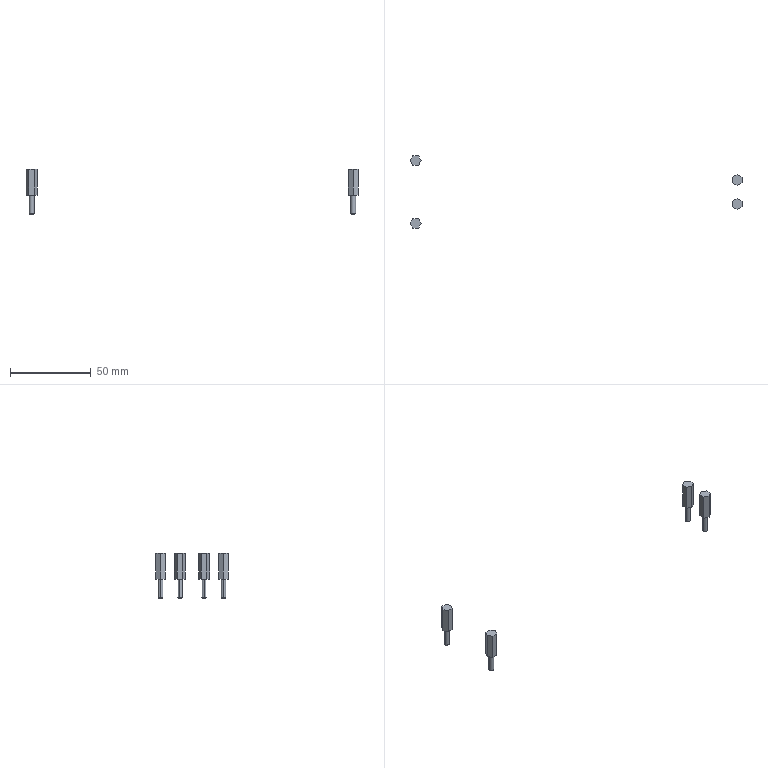Part | SolidWorks | features Chamfer 4, Extrusion 1, ICE 1 | 4 solids | 52 faces | box 205.964 x 45 x 28 mm | volume 2330 mm3 | plane 36 | cone 8 | cylinder 8 | commonest cylinder face diameters 3 x8
STEP:
#1=CARTESIAN_POINT('',(-83.5,19.5,-12.));
#2=VERTEX_POINT('',#1);
#3=CARTESIAN_POINT('',(-81.5,19.5,-12.));
#4=VERTEX_POINT('',#3);
#5=CARTESIAN_POINT('',(-82.5,19.5,-12.));
#6=DIRECTION('',(0.,0.,-1.));
#7=DIRECTION('',(1.,0.,0.));
#8=AXIS2_PLACEMENT_3D('',#5,#6,#7);
#9=CIRCLE('',#8,1.);
#10=EDGE_CURVE('',#2,#4,#9,.T.);
#11=ORIENTED_EDGE('',*,*,#10,.F.);
#12=CARTESIAN_POINT('',(-84.,19.5,-11.5));
#13=VERTEX_POINT('',#12);
#14=CARTESIAN_POINT('',(-84.,19.5,-11.5));
#15=DIRECTION('',(-0.7071,0.,0.7071));
#16=VECTOR('',#15,1000.);
#17=LINE('',#14,#16);
#18=EDGE_CURVE('',#2,#13,#17,.T.);
#19=ORIENTED_EDGE('',*,*,#18,.T.);
#20=CARTESIAN_POINT('',(-81.,19.5,-11.5));
#21=VERTEX_POINT('',#20);
#22=CARTESIAN_POINT('',(-82.5,19.5,-11.5));
#23=DIRECTION('',(0.,0.,1.));
#24=DIRECTION('',(1.,0.,0.));
#25=AXIS2_PLACEMENT_3D('',#22,#23,#24);
#26=CIRCLE('',#25,1.5);
#27=EDGE_CURVE('',#21,#13,#26,.T.);
#28=ORIENTED_EDGE('',*,*,#27,.F.);
#29=CARTESIAN_POINT('',(-81.,19.5,-11.5));
#30=DIRECTION('',(0.7071,0.,0.7071));
#31=VECTOR('',#30,1000.);
#32=LINE('',#29,#31);
#33=EDGE_CURVE('',#4,#21,#32,.T.);
#34=ORIENTED_EDGE('',*,*,#33,.F.);
#35=EDGE_LOOP('',(#11,#19,#28,#34));
#36=FACE_OUTER_BOUND('',#35,.T.);
#37=CARTESIAN_POINT('',(-82.5,19.5,-11.5));
#38=DIRECTION('',(0.,0.,1.));
#39=DIRECTION('',(1.,0.,0.));
#40=AXIS2_PLACEMENT_3D('',#37,#38,#39);
#41=CONICAL_SURFACE('',#40,1.5,0.7854);
#42=ADVANCED_FACE('',(#36),#41,.T.);
#43=ORIENTED_EDGE('',*,*,#27,.T.);
#44=CARTESIAN_POINT('',(-84.,19.5,0.));
#45=VERTEX_POINT('',#44);
#46=CARTESIAN_POINT('',(-84.,19.5,-12.));
#47=DIRECTION('',(0.,0.,1.));
#48=VECTOR('',#47,1000.);
#49=LINE('',#46,#48);
#50=EDGE_CURVE('',#13,#45,#49,.T.);
#51=ORIENTED_EDGE('',*,*,#50,.T.);
#52=CARTESIAN_POINT('',(-81.,19.5,0.));
#53=VERTEX_POINT('',#52);
#54=CARTESIAN_POINT('',(-82.5,19.5,0.));
#55=DIRECTION('',(0.,0.,1.));
#56=DIRECTION('',(1.,0.,0.));
#57=AXIS2_PLACEMENT_3D('',#54,#55,#56);
#58=CIRCLE('',#57,1.5);
#59=EDGE_CURVE('',#53,#45,#58,.T.);
#60=ORIENTED_EDGE('',*,*,#59,.F.);
#61=CARTESIAN_POINT('',(-81.,19.5,-12.));
#62=DIRECTION('',(0.,0.,1.));
#63=VECTOR('',#62,1000.);
#64=LINE('',#61,#63);
#65=EDGE_CURVE('',#21,#53,#64,.T.);
#66=ORIENTED_EDGE('',*,*,#65,.F.);
#67=EDGE_LOOP('',(#43,#51,#60,#66));
#68=FACE_OUTER_BOUND('',#67,.T.);
#69=CARTESIAN_POINT('',(-82.5,19.5,-12.));
#70=DIRECTION('',(0.,0.,1.));
#71=DIRECTION('',(1.,0.,0.));
#72=AXIS2_PLACEMENT_3D('',#69,#70,#71);
#73=CYLINDRICAL_SURFACE('',#72,1.5);
#74=ADVANCED_FACE('',(#68),#73,.T.);
#75=CARTESIAN_POINT('',(-84.232,16.5,0.));
#76=VERTEX_POINT('',#75);
#77=CARTESIAN_POINT('',(-85.964,19.5,0.));
#78=VERTEX_POINT('',#77);
#79=CARTESIAN_POINT('',(-84.232,16.5,0.));
#80=DIRECTION('',(-0.5,0.866,0.));
#81=VECTOR('',#80,1000.);
#82=LINE('',#79,#81);
#83=EDGE_CURVE('',#76,#78,#82,.T.);
#84=ORIENTED_EDGE('',*,*,#83,.F.);
#85=CARTESIAN_POINT('',(-84.232,16.5,16.));
#86=VERTEX_POINT('',#85);
#87=CARTESIAN_POINT('',(-84.232,16.5,16.));
#88=DIRECTION('',(0.,0.,-1.));
#89=VECTOR('',#88,1000.);
#90=LINE('',#87,#89);
#91=EDGE_CURVE('',#86,#76,#90,.T.);
#92=ORIENTED_EDGE('',*,*,#91,.F.);
#93=CARTESIAN_POINT('',(-85.964,19.5,16.));
#94=VERTEX_POINT('',#93);
#95=CARTESIAN_POINT('',(-84.232,16.5,16.));
#96=DIRECTION('',(-0.5,0.866,0.));
#97=VECTOR('',#96,1000.);
#98=LINE('',#95,#97);
#99=EDGE_CURVE('',#86,#94,#98,.T.);
#100=ORIENTED_EDGE('',*,*,#99,.T.);
#101=CARTESIAN_POINT('',(-85.964,19.5,16.));
#102=DIRECTION('',(0.,0.,-1.));
#103=VECTOR('',#102,1000.);
#104=LINE('',#101,#103);
#105=EDGE_CURVE('',#94,#78,#104,.T.);
#106=ORIENTED_EDGE('',*,*,#105,.T.);
#107=EDGE_LOOP('',(#84,#92,#100,#106));
#108=FACE_OUTER_BOUND('',#107,.T.);
#109=CARTESIAN_POINT('',(-84.232,16.5,16.));
#110=DIRECTION('',(-0.866,-0.5,0.));
#111=DIRECTION('',(0.5,-0.866,0.));
#112=AXIS2_PLACEMENT_3D('',#109,#110,#111);
#113=PLANE('',#112);
#114=ADVANCED_FACE('',(#108),#113,.T.);
#115=CARTESIAN_POINT('',(-80.768,16.5,0.));
#116=VERTEX_POINT('',#115);
#117=CARTESIAN_POINT('',(-80.768,16.5,0.));
#118=DIRECTION('',(-1.,0.,0.));
#119=VECTOR('',#118,1000.);
#120=LINE('',#117,#119);
#121=EDGE_CURVE('',#116,#76,#120,.T.);
#122=ORIENTED_EDGE('',*,*,#121,.F.);
#123=CARTESIAN_POINT('',(-80.768,16.5,16.));
#124=VERTEX_POINT('',#123);
#125=CARTESIAN_POINT('',(-80.768,16.5,16.));
#126=DIRECTION('',(0.,0.,-1.));
#127=VECTOR('',#126,1000.);
#128=LINE('',#125,#127);
#129=EDGE_CURVE('',#124,#116,#128,.T.);
#130=ORIENTED_EDGE('',*,*,#129,.F.);
#131=CARTESIAN_POINT('',(-80.768,16.5,16.));
#132=DIRECTION('',(-1.,0.,0.));
#133=VECTOR('',#132,1000.);
#134=LINE('',#131,#133);
#135=EDGE_CURVE('',#124,#86,#134,.T.);
#136=ORIENTED_EDGE('',*,*,#135,.T.);
#137=ORIENTED_EDGE('',*,*,#91,.T.);
#138=EDGE_LOOP('',(#122,#130,#136,#137));
#139=FACE_OUTER_BOUND('',#138,.T.);
#140=CARTESIAN_POINT('',(-80.768,16.5,16.));
#141=DIRECTION('',(0.,-1.,0.));
#142=DIRECTION('',(0.,0.,-1.));
#143=AXIS2_PLACEMENT_3D('',#140,#141,#142);
#144=PLANE('',#143);
#145=ADVANCED_FACE('',(#139),#144,.T.);
#146=CARTESIAN_POINT('',(-79.036,19.5,0.));
#147=VERTEX_POINT('',#146);
#148=CARTESIAN_POINT('',(-79.036,19.5,0.));
#149=DIRECTION('',(-0.5,-0.866,0.));
#150=VECTOR('',#149,1000.);
#151=LINE('',#148,#150);
#152=EDGE_CURVE('',#147,#116,#151,.T.);
#153=ORIENTED_EDGE('',*,*,#152,.F.);
#154=CARTESIAN_POINT('',(-79.036,19.5,16.));
#155=VERTEX_POINT('',#154);
#156=CARTESIAN_POINT('',(-79.036,19.5,16.));
#157=DIRECTION('',(0.,0.,-1.));
#158=VECTOR('',#157,1000.);
#159=LINE('',#156,#158);
#160=EDGE_CURVE('',#155,#147,#159,.T.);
#161=ORIENTED_EDGE('',*,*,#160,.F.);
#162=CARTESIAN_POINT('',(-79.036,19.5,16.));
#163=DIRECTION('',(-0.5,-0.866,0.));
#164=VECTOR('',#163,1000.);
#165=LINE('',#162,#164);
#166=EDGE_CURVE('',#155,#124,#165,.T.);
#167=ORIENTED_EDGE('',*,*,#166,.T.);
#168=ORIENTED_EDGE('',*,*,#129,.T.);
#169=EDGE_LOOP('',(#153,#161,#167,#168));
#170=FACE_OUTER_BOUND('',#169,.T.);
#171=CARTESIAN_POINT('',(-79.036,19.5,16.));
#172=DIRECTION('',(0.866,-0.5,0.));
#173=DIRECTION('',(0.5,0.866,0.));
#174=AXIS2_PLACEMENT_3D('',#171,#172,#173);
#175=PLANE('',#174);
#176=ADVANCED_FACE('',(#170),#175,.T.);
#177=CARTESIAN_POINT('',(-80.768,22.5,0.));
#178=VERTEX_POINT('',#177);
#179=CARTESIAN_POINT('',(-80.768,22.5,0.));
#180=DIRECTION('',(0.5,-0.866,0.));
#181=VECTOR('',#180,1000.);
#182=LINE('',#179,#181);
#183=EDGE_CURVE('',#178,#147,#182,.T.);
#184=ORIENTED_EDGE('',*,*,#183,.F.);
#185=CARTESIAN_POINT('',(-80.768,22.5,16.));
#186=VERTEX_POINT('',#185);
#187=CARTESIAN_POINT('',(-80.768,22.5,16.));
#188=DIRECTION('',(0.,0.,-1.));
#189=VECTOR('',#188,1000.);
#190=LINE('',#187,#189);
#191=EDGE_CURVE('',#186,#178,#190,.T.);
#192=ORIENTED_EDGE('',*,*,#191,.F.);
#193=CARTESIAN_POINT('',(-80.768,22.5,16.));
#194=DIRECTION('',(0.5,-0.866,0.));
#195=VECTOR('',#194,1000.);
#196=LINE('',#193,#195);
#197=EDGE_CURVE('',#186,#155,#196,.T.);
#198=ORIENTED_EDGE('',*,*,#197,.T.);
#199=ORIENTED_EDGE('',*,*,#160,.T.);
#200=EDGE_LOOP('',(#184,#192,#198,#199));
#201=FACE_OUTER_BOUND('',#200,.T.);
#202=CARTESIAN_POINT('',(-80.768,22.5,16.));
#203=DIRECTION('',(0.866,0.5,0.));
#204=DIRECTION('',(-0.5,0.866,0.));
#205=AXIS2_PLACEMENT_3D('',#202,#203,#204);
#206=PLANE('',#205);
#207=ADVANCED_FACE('',(#201),#206,.T.);
#208=CARTESIAN_POINT('',(-84.232,22.5,0.));
#209=VERTEX_POINT('',#208);
#210=CARTESIAN_POINT('',(-84.232,22.5,0.));
#211=DIRECTION('',(1.,0.,0.));
#212=VECTOR('',#211,1000.);
#213=LINE('',#210,#212);
#214=EDGE_CURVE('',#209,#178,#213,.T.);
#215=ORIENTED_EDGE('',*,*,#214,.F.);
#216=CARTESIAN_POINT('',(-84.232,22.5,16.));
#217=VERTEX_POINT('',#216);
#218=CARTESIAN_POINT('',(-84.232,22.5,16.));
#219=DIRECTION('',(0.,0.,-1.));
#220=VECTOR('',#219,1000.);
#221=LINE('',#218,#220);
#222=EDGE_CURVE('',#217,#209,#221,.T.);
#223=ORIENTED_EDGE('',*,*,#222,.F.);
#224=CARTESIAN_POINT('',(-84.232,22.5,16.));
#225=DIRECTION('',(1.,0.,0.));
#226=VECTOR('',#225,1000.);
#227=LINE('',#224,#226);
#228=EDGE_CURVE('',#217,#186,#227,.T.);
#229=ORIENTED_EDGE('',*,*,#228,.T.);
#230=ORIENTED_EDGE('',*,*,#191,.T.);
#231=EDGE_LOOP('',(#215,#223,#229,#230));
#232=FACE_OUTER_BOUND('',#231,.T.);
#233=CARTESIAN_POINT('',(-84.232,22.5,16.));
#234=DIRECTION('',(0.,1.,0.));
#235=DIRECTION('',(0.,0.,1.));
#236=AXIS2_PLACEMENT_3D('',#233,#234,#235);
#237=PLANE('',#236);
#238=ADVANCED_FACE('',(#232),#237,.T.);
#239=CARTESIAN_POINT('',(-85.964,19.5,0.));
#240=DIRECTION('',(0.5,0.866,0.));
#241=VECTOR('',#240,1000.);
#242=LINE('',#239,#241);
#243=EDGE_CURVE('',#78,#209,#242,.T.);
#244=ORIENTED_EDGE('',*,*,#243,.F.);
#245=ORIENTED_EDGE('',*,*,#105,.F.);
#246=CARTESIAN_POINT('',(-85.964,19.5,16.));
#247=DIRECTION('',(0.5,0.866,0.));
#248=VECTOR('',#247,1000.);
#249=LINE('',#246,#248);
#250=EDGE_CURVE('',#94,#217,#249,.T.);
#251=ORIENTED_EDGE('',*,*,#250,.T.);
#252=ORIENTED_EDGE('',*,*,#222,.T.);
#253=EDGE_LOOP('',(#244,#245,#251,#252));
#254=FACE_OUTER_BOUND('',#253,.T.);
#255=CARTESIAN_POINT('',(-85.964,19.5,16.));
#256=DIRECTION('',(-0.866,0.5,0.));
#257=DIRECTION('',(-0.5,-0.866,0.));
#258=AXIS2_PLACEMENT_3D('',#255,#256,#257);
#259=PLANE('',#258);
#260=ADVANCED_FACE('',(#254),#259,.T.);
#261=ORIENTED_EDGE('',*,*,#99,.F.);
#262=ORIENTED_EDGE('',*,*,#135,.F.);
#263=ORIENTED_EDGE('',*,*,#166,.F.);
#264=ORIENTED_EDGE('',*,*,#197,.F.);
#265=ORIENTED_EDGE('',*,*,#228,.F.);
#266=ORIENTED_EDGE('',*,*,#250,.F.);
#267=EDGE_LOOP('',(#261,#262,#263,#264,#265,#266));
#268=FACE_OUTER_BOUND('',#267,.T.);
#269=CARTESIAN_POINT('',(0.,0.,16.));
#270=DIRECTION('',(0.,0.,-1.));
#271=DIRECTION('',(-1.,0.,0.));
#272=AXIS2_PLACEMENT_3D('',#269,#270,#271);
#273=PLANE('',#272);
#274=ADVANCED_FACE('',(#268),#273,.F.);
#275=ORIENTED_EDGE('',*,*,#59,.T.);
#276=CARTESIAN_POINT('',(-82.5,19.5,0.));
#277=DIRECTION('',(0.,0.,1.));
#278=DIRECTION('',(1.,0.,0.));
#279=AXIS2_PLACEMENT_3D('',#276,#277,#278);
#280=CIRCLE('',#279,1.5);
#281=EDGE_CURVE('',#45,#53,#280,.T.);
#282=ORIENTED_EDGE('',*,*,#281,.T.);
#283=EDGE_LOOP('',(#275,#282));
#284=FACE_BOUND('',#283,.T.);
#285=ORIENTED_EDGE('',*,*,#83,.T.);
#286=ORIENTED_EDGE('',*,*,#243,.T.);
#287=ORIENTED_EDGE('',*,*,#214,.T.);
#288=ORIENTED_EDGE('',*,*,#183,.T.);
#289=ORIENTED_EDGE('',*,*,#152,.T.);
#290=ORIENTED_EDGE('',*,*,#121,.T.);
#291=EDGE_LOOP('',(#285,#286,#287,#288,#289,#290));
#292=FACE_OUTER_BOUND('',#291,.T.);
#293=CARTESIAN_POINT('',(0.,0.,0.));
#294=DIRECTION('',(0.,0.,-1.));
#295=DIRECTION('',(-1.,0.,0.));
#296=AXIS2_PLACEMENT_3D('',#293,#294,#295);
#297=PLANE('',#296);
#298=ADVANCED_FACE('',(#284,#292),#297,.T.);
#299=ORIENTED_EDGE('',*,*,#50,.F.);
#300=CARTESIAN_POINT('',(-82.5,19.5,-11.5));
#301=DIRECTION('',(0.,0.,1.));
#302=DIRECTION('',(1.,0.,0.));
#303=AXIS2_PLACEMENT_3D('',#300,#301,#302);
#304=CIRCLE('',#303,1.5);
#305=EDGE_CURVE('',#13,#21,#304,.T.);
#306=ORIENTED_EDGE('',*,*,#305,.T.);
#307=ORIENTED_EDGE('',*,*,#65,.T.);
#308=ORIENTED_EDGE('',*,*,#281,.F.);
#309=EDGE_LOOP('',(#299,#306,#307,#308));
#310=FACE_OUTER_BOUND('',#309,.T.);
#311=CARTESIAN_POINT('',(-82.5,19.5,-12.));
#312=DIRECTION('',(0.,0.,1.));
#313=DIRECTION('',(1.,0.,0.));
#314=AXIS2_PLACEMENT_3D('',#311,#312,#313);
#315=CYLINDRICAL_SURFACE('',#314,1.5);
#316=ADVANCED_FACE('',(#310),#315,.T.);
#317=CARTESIAN_POINT('',(-82.5,19.5,-12.));
#318=DIRECTION('',(0.,0.,-1.));
#319=DIRECTION('',(1.,0.,0.));
#320=AXIS2_PLACEMENT_3D('',#317,#318,#319);
#321=CIRCLE('',#320,1.);
#322=EDGE_CURVE('',#4,#2,#321,.T.);
#323=ORIENTED_EDGE('',*,*,#322,.T.);
#324=ORIENTED_EDGE('',*,*,#10,.T.);
#325=EDGE_LOOP('',(#323,#324));
#326=FACE_OUTER_BOUND('',#325,.T.);
#327=CARTESIAN_POINT('',(-82.5,19.5,-12.));
#328=DIRECTION('',(0.,0.,1.));
#329=DIRECTION('',(1.,0.,0.));
#330=AXIS2_PLACEMENT_3D('',#327,#328,#329);
#331=PLANE('',#330);
#332=ADVANCED_FACE('',(#326),#331,.F.);
#333=ORIENTED_EDGE('',*,*,#18,.F.);
#334=ORIENTED_EDGE('',*,*,#322,.F.);
#335=ORIENTED_EDGE('',*,*,#33,.T.);
#336=ORIENTED_EDGE('',*,*,#305,.F.);
#337=EDGE_LOOP('',(#333,#334,#335,#336));
#338=FACE_OUTER_BOUND('',#337,.T.);
#339=CARTESIAN_POINT('',(-82.5,19.5,-11.5));
#340=DIRECTION('',(0.,0.,1.));
#341=DIRECTION('',(1.,0.,0.));
#342=AXIS2_PLACEMENT_3D('',#339,#340,#341);
#343=CONICAL_SURFACE('',#342,1.5,0.7854);
#344=ADVANCED_FACE('',(#338),#343,.T.);
#345=CLOSED_SHELL('',(#42,#74,#114,#145,#176,#207,#238,#260,#274,#298,#316,#332,#344));
#346=MANIFOLD_SOLID_BREP('',#345);
#347=CARTESIAN_POINT('',(-83.5,-19.5,-12.));
#348=VERTEX_POINT('',#347);
#349=CARTESIAN_POINT('',(-81.5,-19.5,-12.));
#350=VERTEX_POINT('',#349);
#351=CARTESIAN_POINT('',(-82.5,-19.5,-12.));
#352=DIRECTION('',(0.,0.,-1.));
#353=DIRECTION('',(1.,0.,0.));
#354=AXIS2_PLACEMENT_3D('',#351,#352,#353);
#355=CIRCLE('',#354,1.);
#356=EDGE_CURVE('',#348,#350,#355,.T.);
#357=ORIENTED_EDGE('',*,*,#356,.F.);
#358=CARTESIAN_POINT('',(-84.,-19.5,-11.5));
#359=VERTEX_POINT('',#358);
#360=CARTESIAN_POINT('',(-84.,-19.5,-11.5));
#361=DIRECTION('',(-0.7071,0.,0.7071));
#362=VECTOR('',#361,1000.);
#363=LINE('',#360,#362);
#364=EDGE_CURVE('',#348,#359,#363,.T.);
#365=ORIENTED_EDGE('',*,*,#364,.T.);
#366=CARTESIAN_POINT('',(-81.,-19.5,-11.5));
#367=VERTEX_POINT('',#366);
#368=CARTESIAN_POINT('',(-82.5,-19.5,-11.5));
#369=DIRECTION('',(0.,0.,1.));
#370=DIRECTION('',(1.,0.,0.));
#371=AXIS2_PLACEMENT_3D('',#368,#369,#370);
#372=CIRCLE('',#371,1.5);
#373=EDGE_CURVE('',#367,#359,#372,.T.);
#374=ORIENTED_EDGE('',*,*,#373,.F.);
#375=CARTESIAN_POINT('',(-81.,-19.5,-11.5));
#376=DIRECTION('',(0.7071,0.,0.7071));
#377=VECTOR('',#376,1000.);
#378=LINE('',#375,#377);
#379=EDGE_CURVE('',#350,#367,#378,.T.);
#380=ORIENTED_EDGE('',*,*,#379,.F.);
#381=EDGE_LOOP('',(#357,#365,#374,#380));
#382=FACE_OUTER_BOUND('',#381,.T.);
#383=CARTESIAN_POINT('',(-82.5,-19.5,-11.5));
#384=DIRECTION('',(0.,0.,1.));
#385=DIRECTION('',(1.,0.,0.));
#386=AXIS2_PLACEMENT_3D('',#383,#384,#385);
#387=CONICAL_SURFACE('',#386,1.5,0.7854);
#388=ADVANCED_FACE('',(#382),#387,.T.);
#389=ORIENTED_EDGE('',*,*,#373,.T.);
#390=CARTESIAN_POINT('',(-84.,-19.5,0.));
#391=VERTEX_POINT('',#390);
#392=CARTESIAN_POINT('',(-84.,-19.5,-12.));
#393=DIRECTION('',(0.,0.,1.));
#394=VECTOR('',#393,1000.);
#395=LINE('',#392,#394);
#396=EDGE_CURVE('',#359,#391,#395,.T.);
#397=ORIENTED_EDGE('',*,*,#396,.T.);
#398=CARTESIAN_POINT('',(-81.,-19.5,0.));
#399=VERTEX_POINT('',#398);
#400=CARTESIAN_POINT('',(-82.5,-19.5,0.));
#401=DIRECTION('',(0.,0.,1.));
#402=DIRECTION('',(1.,0.,0.));
#403=AXIS2_PLACEMENT_3D('',#400,#401,#402);
#404=CIRCLE('',#403,1.5);
#405=EDGE_CURVE('',#399,#391,#404,.T.);
#406=ORIENTED_EDGE('',*,*,#405,.F.);
#407=CARTESIAN_POINT('',(-81.,-19.5,-12.));
#408=DIRECTION('',(0.,0.,1.));
#409=VECTOR('',#408,1000.);
#410=LINE('',#407,#409);
#411=EDGE_CURVE('',#367,#399,#410,.T.);
#412=ORIENTED_EDGE('',*,*,#411,.F.);
#413=EDGE_LOOP('',(#389,#397,#406,#412));
#414=FACE_OUTER_BOUND('',#413,.T.);
#415=CARTESIAN_POINT('',(-82.5,-19.5,-12.));
#416=DIRECTION('',(0.,0.,1.));
#417=DIRECTION('',(1.,0.,0.));
#418=AXIS2_PLACEMENT_3D('',#415,#416,#417);
#419=CYLINDRICAL_SURFACE('',#418,1.5);
#420=ADVANCED_FACE('',(#414),#419,.T.);
#421=CARTESIAN_POINT('',(-79.036,-19.5,0.));
#422=VERTEX_POINT('',#421);
#423=CARTESIAN_POINT('',(-80.768,-16.5,0.));
#424=VERTEX_POINT('',#423);
#425=CARTESIAN_POINT('',(-79.036,-19.5,0.));
#426=DIRECTION('',(-0.5,0.866,0.));
#427=VECTOR('',#426,1000.);
#428=LINE('',#425,#427);
#429=EDGE_CURVE('',#422,#424,#428,.T.);
#430=ORIENTED_EDGE('',*,*,#429,.T.);
#431=CARTESIAN_POINT('',(-80.768,-16.5,16.));
#432=VERTEX_POINT('',#431);
#433=CARTESIAN_POINT('',(-80.768,-16.5,16.));
#434=DIRECTION('',(0.,0.,-1.));
#435=VECTOR('',#434,1000.);
#436=LINE('',#433,#435);
#437=EDGE_CURVE('',#432,#424,#436,.T.);
#438=ORIENTED_EDGE('',*,*,#437,.F.);
#439=CARTESIAN_POINT('',(-79.036,-19.5,16.));
#440=VERTEX_POINT('',#439);
#441=CARTESIAN_POINT('',(-79.036,-19.5,16.));
#442=DIRECTION('',(-0.5,0.866,0.));
#443=VECTOR('',#442,1000.);
#444=LINE('',#441,#443);
#445=EDGE_CURVE('',#440,#432,#444,.T.);
#446=ORIENTED_EDGE('',*,*,#445,.F.);
#447=CARTESIAN_POINT('',(-79.036,-19.5,16.));
#448=DIRECTION('',(0.,0.,-1.));
#449=VECTOR('',#448,1000.);
#450=LINE('',#447,#449);
#451=EDGE_CURVE('',#440,#422,#450,.T.);
#452=ORIENTED_EDGE('',*,*,#451,.T.);
#453=EDGE_LOOP('',(#430,#438,#446,#452));
#454=FACE_OUTER_BOUND('',#453,.T.);
#455=CARTESIAN_POINT('',(-79.036,-19.5,16.));
#456=DIRECTION('',(-0.866,-0.5,0.));
#457=DIRECTION('',(0.5,-0.866,0.));
#458=AXIS2_PLACEMENT_3D('',#455,#456,#457);
#459=PLANE('',#458);
#460=ADVANCED_FACE('',(#454),#459,.F.);
#461=CARTESIAN_POINT('',(-84.232,-16.5,0.));
#462=VERTEX_POINT('',#461);
#463=CARTESIAN_POINT('',(-80.768,-16.5,0.));
#464=DIRECTION('',(-1.,0.,0.));
#465=VECTOR('',#464,1000.);
#466=LINE('',#463,#465);
#467=EDGE_CURVE('',#424,#462,#466,.T.);
#468=ORIENTED_EDGE('',*,*,#467,.T.);
#469=CARTESIAN_POINT('',(-84.232,-16.5,16.));
#470=VERTEX_POINT('',#469);
#471=CARTESIAN_POINT('',(-84.232,-16.5,16.));
#472=DIRECTION('',(0.,0.,-1.));
#473=VECTOR('',#472,1000.);
#474=LINE('',#471,#473);
#475=EDGE_CURVE('',#470,#462,#474,.T.);
#476=ORIENTED_EDGE('',*,*,#475,.F.);
#477=CARTESIAN_POINT('',(-80.768,-16.5,16.));
#478=DIRECTION('',(-1.,0.,0.));
#479=VECTOR('',#478,1000.);
#480=LINE('',#477,#479);
#481=EDGE_CURVE('',#432,#470,#480,.T.);
#482=ORIENTED_EDGE('',*,*,#481,.F.);
#483=ORIENTED_EDGE('',*,*,#437,.T.);
#484=EDGE_LOOP('',(#468,#476,#482,#483));
#485=FACE_OUTER_BOUND('',#484,.T.);
#486=CARTESIAN_POINT('',(-80.768,-16.5,16.));
#487=DIRECTION('',(0.,-1.,0.));
#488=DIRECTION('',(0.,0.,-1.));
#489=AXIS2_PLACEMENT_3D('',#486,#487,#488);
#490=PLANE('',#489);
#491=ADVANCED_FACE('',(#485),#490,.F.);
#492=CARTESIAN_POINT('',(-85.964,-19.5,0.));
#493=VERTEX_POINT('',#492);
#494=CARTESIAN_POINT('',(-84.232,-16.5,0.));
#495=DIRECTION('',(-0.5,-0.866,0.));
#496=VECTOR('',#495,1000.);
#497=LINE('',#494,#496);
#498=EDGE_CURVE('',#462,#493,#497,.T.);
#499=ORIENTED_EDGE('',*,*,#498,.T.);
#500=CARTESIAN_POINT('',(-85.964,-19.5,16.));
#501=VERTEX_POINT('',#500);
#502=CARTESIAN_POINT('',(-85.964,-19.5,16.));
#503=DIRECTION('',(0.,0.,-1.));
#504=VECTOR('',#503,1000.);
#505=LINE('',#502,#504);
#506=EDGE_CURVE('',#501,#493,#505,.T.);
#507=ORIENTED_EDGE('',*,*,#506,.F.);
#508=CARTESIAN_POINT('',(-84.232,-16.5,16.));
#509=DIRECTION('',(-0.5,-0.866,0.));
#510=VECTOR('',#509,1000.);
#511=LINE('',#508,#510);
#512=EDGE_CURVE('',#470,#501,#511,.T.);
#513=ORIENTED_EDGE('',*,*,#512,.F.);
#514=ORIENTED_EDGE('',*,*,#475,.T.);
#515=EDGE_LOOP('',(#499,#507,#513,#514));
#516=FACE_OUTER_BOUND('',#515,.T.);
#517=CARTESIAN_POINT('',(-84.232,-16.5,16.));
#518=DIRECTION('',(0.866,-0.5,0.));
#519=DIRECTION('',(0.5,0.866,0.));
#520=AXIS2_PLACEMENT_3D('',#517,#518,#519);
#521=PLANE('',#520);
#522=ADVANCED_FACE('',(#516),#521,.F.);
#523=CARTESIAN_POINT('',(-84.232,-22.5,0.));
#524=VERTEX_POINT('',#523);
#525=CARTESIAN_POINT('',(-85.964,-19.5,0.));
#526=DIRECTION('',(0.5,-0.866,0.));
#527=VECTOR('',#526,1000.);
#528=LINE('',#525,#527);
#529=EDGE_CURVE('',#493,#524,#528,.T.);
#530=ORIENTED_EDGE('',*,*,#529,.T.);
#531=CARTESIAN_POINT('',(-84.232,-22.5,16.));
#532=VERTEX_POINT('',#531);
#533=CARTESIAN_POINT('',(-84.232,-22.5,16.));
#534=DIRECTION('',(0.,0.,-1.));
#535=VECTOR('',#534,1000.);
#536=LINE('',#533,#535);
#537=EDGE_CURVE('',#532,#524,#536,.T.);
#538=ORIENTED_EDGE('',*,*,#537,.F.);
#539=CARTESIAN_POINT('',(-85.964,-19.5,16.));
#540=DIRECTION('',(0.5,-0.866,0.));
#541=VECTOR('',#540,1000.);
#542=LINE('',#539,#541);
#543=EDGE_CURVE('',#501,#532,#542,.T.);
#544=ORIENTED_EDGE('',*,*,#543,.F.);
#545=ORIENTED_EDGE('',*,*,#506,.T.);
#546=EDGE_LOOP('',(#530,#538,#544,#545));
#547=FACE_OUTER_BOUND('',#546,.T.);
#548=CARTESIAN_POINT('',(-85.964,-19.5,16.));
#549=DIRECTION('',(0.866,0.5,0.));
#550=DIRECTION('',(-0.5,0.866,0.));
#551=AXIS2_PLACEMENT_3D('',#548,#549,#550);
#552=PLANE('',#551);
#553=ADVANCED_FACE('',(#547),#552,.F.);
#554=CARTESIAN_POINT('',(-80.768,-22.5,0.));
#555=VERTEX_POINT('',#554);
#556=CARTESIAN_POINT('',(-84.232,-22.5,0.));
#557=DIRECTION('',(1.,0.,0.));
#558=VECTOR('',#557,1000.);
#559=LINE('',#556,#558);
#560=EDGE_CURVE('',#524,#555,#559,.T.);
#561=ORIENTED_EDGE('',*,*,#560,.T.);
#562=CARTESIAN_POINT('',(-80.768,-22.5,16.));
#563=VERTEX_POINT('',#562);
#564=CARTESIAN_POINT('',(-80.768,-22.5,16.));
#565=DIRECTION('',(0.,0.,-1.));
#566=VECTOR('',#565,1000.);
#567=LINE('',#564,#566);
#568=EDGE_CURVE('',#563,#555,#567,.T.);
#569=ORIENTED_EDGE('',*,*,#568,.F.);
#570=CARTESIAN_POINT('',(-84.232,-22.5,16.));
#571=DIRECTION('',(1.,0.,0.));
#572=VECTOR('',#571,1000.);
#573=LINE('',#570,#572);
#574=EDGE_CURVE('',#532,#563,#573,.T.);
#575=ORIENTED_EDGE('',*,*,#574,.F.);
#576=ORIENTED_EDGE('',*,*,#537,.T.);
#577=EDGE_LOOP('',(#561,#569,#575,#576));
#578=FACE_OUTER_BOUND('',#577,.T.);
#579=CARTESIAN_POINT('',(-84.232,-22.5,16.));
#580=DIRECTION('',(0.,1.,0.));
#581=DIRECTION('',(0.,0.,1.));
#582=AXIS2_PLACEMENT_3D('',#579,#580,#581);
#583=PLANE('',#582);
#584=ADVANCED_FACE('',(#578),#583,.F.);
#585=CARTESIAN_POINT('',(-80.768,-22.5,0.));
#586=DIRECTION('',(0.5,0.866,0.));
#587=VECTOR('',#586,1000.);
#588=LINE('',#585,#587);
#589=EDGE_CURVE('',#555,#422,#588,.T.);
#590=ORIENTED_EDGE('',*,*,#589,.T.);
#591=ORIENTED_EDGE('',*,*,#451,.F.);
#592=CARTESIAN_POINT('',(-80.768,-22.5,16.));
#593=DIRECTION('',(0.5,0.866,0.));
#594=VECTOR('',#593,1000.);
#595=LINE('',#592,#594);
#596=EDGE_CURVE('',#563,#440,#595,.T.);
#597=ORIENTED_EDGE('',*,*,#596,.F.);
#598=ORIENTED_EDGE('',*,*,#568,.T.);
#599=EDGE_LOOP('',(#590,#591,#597,#598));
#600=FACE_OUTER_BOUND('',#599,.T.);
#601=CARTESIAN_POINT('',(-80.768,-22.5,16.));
#602=DIRECTION('',(-0.866,0.5,0.));
#603=DIRECTION('',(-0.5,-0.866,0.));
#604=AXIS2_PLACEMENT_3D('',#601,#602,#603);
#605=PLANE('',#604);
#606=ADVANCED_FACE('',(#600),#605,.F.);
#607=ORIENTED_EDGE('',*,*,#445,.T.);
#608=ORIENTED_EDGE('',*,*,#481,.T.);
#609=ORIENTED_EDGE('',*,*,#512,.T.);
#610=ORIENTED_EDGE('',*,*,#543,.T.);
#611=ORIENTED_EDGE('',*,*,#574,.T.);
#612=ORIENTED_EDGE('',*,*,#596,.T.);
#613=EDGE_LOOP('',(#607,#608,#609,#610,#611,#612));
#614=FACE_OUTER_BOUND('',#613,.T.);
#615=CARTESIAN_POINT('',(0.,0.,16.));
#616=DIRECTION('',(0.,0.,1.));
#617=DIRECTION('',(1.,0.,0.));
#618=AXIS2_PLACEMENT_3D('',#615,#616,#617);
#619=PLANE('',#618);
#620=ADVANCED_FACE('',(#614),#619,.T.);
#621=ORIENTED_EDGE('',*,*,#405,.T.);
#622=CARTESIAN_POINT('',(-82.5,-19.5,0.));
#623=DIRECTION('',(0.,0.,1.));
#624=DIRECTION('',(1.,0.,0.));
#625=AXIS2_PLACEMENT_3D('',#622,#623,#624);
#626=CIRCLE('',#625,1.5);
#627=EDGE_CURVE('',#391,#399,#626,.T.);
#628=ORIENTED_EDGE('',*,*,#627,.T.);
#629=EDGE_LOOP('',(#621,#628));
#630=FACE_BOUND('',#629,.T.);
#631=ORIENTED_EDGE('',*,*,#429,.F.);
#632=ORIENTED_EDGE('',*,*,#589,.F.);
#633=ORIENTED_EDGE('',*,*,#560,.F.);
#634=ORIENTED_EDGE('',*,*,#529,.F.);
#635=ORIENTED_EDGE('',*,*,#498,.F.);
#636=ORIENTED_EDGE('',*,*,#467,.F.);
#637=EDGE_LOOP('',(#631,#632,#633,#634,#635,#636));
#638=FACE_OUTER_BOUND('',#637,.T.);
#639=CARTESIAN_POINT('',(0.,0.,0.));
#640=DIRECTION('',(0.,0.,1.));
#641=DIRECTION('',(1.,0.,0.));
#642=AXIS2_PLACEMENT_3D('',#639,#640,#641);
#643=PLANE('',#642);
#644=ADVANCED_FACE('',(#630,#638),#643,.F.);
#645=ORIENTED_EDGE('',*,*,#396,.F.);
#646=CARTESIAN_POINT('',(-82.5,-19.5,-11.5));
#647=DIRECTION('',(0.,0.,1.));
#648=DIRECTION('',(1.,0.,0.));
#649=AXIS2_PLACEMENT_3D('',#646,#647,#648);
#650=CIRCLE('',#649,1.5);
#651=EDGE_CURVE('',#359,#367,#650,.T.);
#652=ORIENTED_EDGE('',*,*,#651,.T.);
#653=ORIENTED_EDGE('',*,*,#411,.T.);
#654=ORIENTED_EDGE('',*,*,#627,.F.);
#655=EDGE_LOOP('',(#645,#652,#653,#654));
#656=FACE_OUTER_BOUND('',#655,.T.);
#657=CARTESIAN_POINT('',(-82.5,-19.5,-12.));
#658=DIRECTION('',(0.,0.,1.));
#659=DIRECTION('',(1.,0.,0.));
#660=AXIS2_PLACEMENT_3D('',#657,#658,#659);
#661=CYLINDRICAL_SURFACE('',#660,1.5);
#662=ADVANCED_FACE('',(#656),#661,.T.);
#663=CARTESIAN_POINT('',(-82.5,-19.5,-12.));
#664=DIRECTION('',(0.,0.,-1.));
#665=DIRECTION('',(1.,0.,0.));
#666=AXIS2_PLACEMENT_3D('',#663,#664,#665);
#667=CIRCLE('',#666,1.);
#668=EDGE_CURVE('',#350,#348,#667,.T.);
#669=ORIENTED_EDGE('',*,*,#668,.T.);
#670=ORIENTED_EDGE('',*,*,#356,.T.);
#671=EDGE_LOOP('',(#669,#670));
#672=FACE_OUTER_BOUND('',#671,.T.);
#673=CARTESIAN_POINT('',(-82.5,-19.5,-12.));
#674=DIRECTION('',(0.,0.,1.));
#675=DIRECTION('',(1.,0.,0.));
#676=AXIS2_PLACEMENT_3D('',#673,#674,#675);
#677=PLANE('',#676);
#678=ADVANCED_FACE('',(#672),#677,.F.);
#679=ORIENTED_EDGE('',*,*,#364,.F.);
#680=ORIENTED_EDGE('',*,*,#668,.F.);
#681=ORIENTED_EDGE('',*,*,#379,.T.);
#682=ORIENTED_EDGE('',*,*,#651,.F.);
#683=EDGE_LOOP('',(#679,#680,#681,#682));
#684=FACE_OUTER_BOUND('',#683,.T.);
#685=CARTESIAN_POINT('',(-82.5,-19.5,-11.5));
#686=DIRECTION('',(0.,0.,1.));
#687=DIRECTION('',(1.,0.,0.));
#688=AXIS2_PLACEMENT_3D('',#685,#686,#687);
#689=CONICAL_SURFACE('',#688,1.5,0.7854);
#690=ADVANCED_FACE('',(#684),#689,.T.);
#691=CLOSED_SHELL('',(#388,#420,#460,#491,#522,#553,#584,#606,#620,#644,#662,#678,#690));
#692=MANIFOLD_SOLID_BREP('',#691);
#693=CARTESIAN_POINT('',(116.,7.5,-12.));
#694=VERTEX_POINT('',#693);
#695=CARTESIAN_POINT('',(118.,7.5,-12.));
#696=VERTEX_POINT('',#695);
#697=CARTESIAN_POINT('',(117.,7.5,-12.));
#698=DIRECTION('',(0.,0.,-1.));
#699=DIRECTION('',(1.,0.,0.));
#700=AXIS2_PLACEMENT_3D('',#697,#698,#699);
#701=CIRCLE('',#700,1.);
#702=EDGE_CURVE('',#694,#696,#701,.T.);
#703=ORIENTED_EDGE('',*,*,#702,.F.);
#704=CARTESIAN_POINT('',(115.5,7.5,-11.5));
#705=VERTEX_POINT('',#704);
#706=CARTESIAN_POINT('',(115.5,7.5,-11.5));
#707=DIRECTION('',(-0.7071,0.,0.7071));
#708=VECTOR('',#707,1000.);
#709=LINE('',#706,#708);
#710=EDGE_CURVE('',#694,#705,#709,.T.);
#711=ORIENTED_EDGE('',*,*,#710,.T.);
#712=CARTESIAN_POINT('',(118.5,7.5,-11.5));
#713=VERTEX_POINT('',#712);
#714=CARTESIAN_POINT('',(117.,7.5,-11.5));
#715=DIRECTION('',(0.,0.,1.));
#716=DIRECTION('',(1.,0.,0.));
#717=AXIS2_PLACEMENT_3D('',#714,#715,#716);
#718=CIRCLE('',#717,1.5);
#719=EDGE_CURVE('',#713,#705,#718,.T.);
#720=ORIENTED_EDGE('',*,*,#719,.F.);
#721=CARTESIAN_POINT('',(118.5,7.5,-11.5));
#722=DIRECTION('',(0.7071,0.,0.7071));
#723=VECTOR('',#722,1000.);
#724=LINE('',#721,#723);
#725=EDGE_CURVE('',#696,#713,#724,.T.);
#726=ORIENTED_EDGE('',*,*,#725,.F.);
#727=EDGE_LOOP('',(#703,#711,#720,#726));
#728=FACE_OUTER_BOUND('',#727,.T.);
#729=CARTESIAN_POINT('',(117.,7.5,-11.5));
#730=DIRECTION('',(0.,0.,1.));
#731=DIRECTION('',(1.,0.,0.));
#732=AXIS2_PLACEMENT_3D('',#729,#730,#731);
#733=CONICAL_SURFACE('',#732,1.5,0.7854);
#734=ADVANCED_FACE('',(#728),#733,.T.);
#735=ORIENTED_EDGE('',*,*,#719,.T.);
#736=CARTESIAN_POINT('',(115.5,7.5,0.));
#737=VERTEX_POINT('',#736);
#738=CARTESIAN_POINT('',(115.5,7.5,-12.));
#739=DIRECTION('',(0.,0.,1.));
#740=VECTOR('',#739,1000.);
#741=LINE('',#738,#740);
#742=EDGE_CURVE('',#705,#737,#741,.T.);
#743=ORIENTED_EDGE('',*,*,#742,.T.);
#744=CARTESIAN_POINT('',(118.5,7.5,0.));
#745=VERTEX_POINT('',#744);
#746=CARTESIAN_POINT('',(117.,7.5,0.));
#747=DIRECTION('',(0.,0.,1.));
#748=DIRECTION('',(1.,0.,0.));
#749=AXIS2_PLACEMENT_3D('',#746,#747,#748);
#750=CIRCLE('',#749,1.5);
#751=EDGE_CURVE('',#745,#737,#750,.T.);
#752=ORIENTED_EDGE('',*,*,#751,.F.);
#753=CARTESIAN_POINT('',(118.5,7.5,-12.));
#754=DIRECTION('',(0.,0.,1.));
#755=VECTOR('',#754,1000.);
#756=LINE('',#753,#755);
#757=EDGE_CURVE('',#713,#745,#756,.T.);
#758=ORIENTED_EDGE('',*,*,#757,.F.);
#759=EDGE_LOOP('',(#735,#743,#752,#758));
#760=FACE_OUTER_BOUND('',#759,.T.);
#761=CARTESIAN_POINT('',(117.,7.5,-12.));
#762=DIRECTION('',(0.,0.,1.));
#763=DIRECTION('',(1.,0.,0.));
#764=AXIS2_PLACEMENT_3D('',#761,#762,#763);
#765=CYLINDRICAL_SURFACE('',#764,1.5);
#766=ADVANCED_FACE('',(#760),#765,.T.);
#767=CARTESIAN_POINT('',(114.,9.232,0.));
#768=VERTEX_POINT('',#767);
#769=CARTESIAN_POINT('',(117.,10.964,0.));
#770=VERTEX_POINT('',#769);
#771=CARTESIAN_POINT('',(114.,9.232,0.));
#772=DIRECTION('',(0.866,0.5,0.));
#773=VECTOR('',#772,1000.);
#774=LINE('',#771,#773);
#775=EDGE_CURVE('',#768,#770,#774,.T.);
#776=ORIENTED_EDGE('',*,*,#775,.F.);
#777=CARTESIAN_POINT('',(114.,9.232,16.));
#778=VERTEX_POINT('',#777);
#779=CARTESIAN_POINT('',(114.,9.232,16.));
#780=DIRECTION('',(0.,0.,-1.));
#781=VECTOR('',#780,1000.);
#782=LINE('',#779,#781);
#783=EDGE_CURVE('',#778,#768,#782,.T.);
#784=ORIENTED_EDGE('',*,*,#783,.F.);
#785=CARTESIAN_POINT('',(117.,10.964,16.));
#786=VERTEX_POINT('',#785);
#787=CARTESIAN_POINT('',(114.,9.232,16.));
#788=DIRECTION('',(0.866,0.5,0.));
#789=VECTOR('',#788,1000.);
#790=LINE('',#787,#789);
#791=EDGE_CURVE('',#778,#786,#790,.T.);
#792=ORIENTED_EDGE('',*,*,#791,.T.);
#793=CARTESIAN_POINT('',(117.,10.964,16.));
#794=DIRECTION('',(0.,0.,-1.));
#795=VECTOR('',#794,1000.);
#796=LINE('',#793,#795);
#797=EDGE_CURVE('',#786,#770,#796,.T.);
#798=ORIENTED_EDGE('',*,*,#797,.T.);
#799=EDGE_LOOP('',(#776,#784,#792,#798));
#800=FACE_OUTER_BOUND('',#799,.T.);
#801=CARTESIAN_POINT('',(114.,9.232,16.));
#802=DIRECTION('',(-0.5,0.866,0.));
#803=DIRECTION('',(-0.866,-0.5,0.));
#804=AXIS2_PLACEMENT_3D('',#801,#802,#803);
#805=PLANE('',#804);
#806=ADVANCED_FACE('',(#800),#805,.T.);
#807=CARTESIAN_POINT('',(114.,5.768,0.));
#808=VERTEX_POINT('',#807);
#809=CARTESIAN_POINT('',(114.,5.768,0.));
#810=DIRECTION('',(0.,1.,0.));
#811=VECTOR('',#810,1000.);
#812=LINE('',#809,#811);
#813=EDGE_CURVE('',#808,#768,#812,.T.);
#814=ORIENTED_EDGE('',*,*,#813,.F.);
#815=CARTESIAN_POINT('',(114.,5.768,16.));
#816=VERTEX_POINT('',#815);
#817=CARTESIAN_POINT('',(114.,5.768,16.));
#818=DIRECTION('',(0.,0.,-1.));
#819=VECTOR('',#818,1000.);
#820=LINE('',#817,#819);
#821=EDGE_CURVE('',#816,#808,#820,.T.);
#822=ORIENTED_EDGE('',*,*,#821,.F.);
#823=CARTESIAN_POINT('',(114.,5.768,16.));
#824=DIRECTION('',(0.,1.,0.));
#825=VECTOR('',#824,1000.);
#826=LINE('',#823,#825);
#827=EDGE_CURVE('',#816,#778,#826,.T.);
#828=ORIENTED_EDGE('',*,*,#827,.T.);
#829=ORIENTED_EDGE('',*,*,#783,.T.);
#830=EDGE_LOOP('',(#814,#822,#828,#829));
#831=FACE_OUTER_BOUND('',#830,.T.);
#832=CARTESIAN_POINT('',(114.,5.768,16.));
#833=DIRECTION('',(-1.,0.,0.));
#834=DIRECTION('',(0.,0.,1.));
#835=AXIS2_PLACEMENT_3D('',#832,#833,#834);
#836=PLANE('',#835);
#837=ADVANCED_FACE('',(#831),#836,.T.);
#838=CARTESIAN_POINT('',(117.,4.036,0.));
#839=VERTEX_POINT('',#838);
#840=CARTESIAN_POINT('',(117.,4.036,0.));
#841=DIRECTION('',(-0.866,0.5,0.));
#842=VECTOR('',#841,1000.);
#843=LINE('',#840,#842);
#844=EDGE_CURVE('',#839,#808,#843,.T.);
#845=ORIENTED_EDGE('',*,*,#844,.F.);
#846=CARTESIAN_POINT('',(117.,4.036,16.));
#847=VERTEX_POINT('',#846);
#848=CARTESIAN_POINT('',(117.,4.036,16.));
#849=DIRECTION('',(0.,0.,-1.));
#850=VECTOR('',#849,1000.);
#851=LINE('',#848,#850);
#852=EDGE_CURVE('',#847,#839,#851,.T.);
#853=ORIENTED_EDGE('',*,*,#852,.F.);
#854=CARTESIAN_POINT('',(117.,4.036,16.));
#855=DIRECTION('',(-0.866,0.5,0.));
#856=VECTOR('',#855,1000.);
#857=LINE('',#854,#856);
#858=EDGE_CURVE('',#847,#816,#857,.T.);
#859=ORIENTED_EDGE('',*,*,#858,.T.);
#860=ORIENTED_EDGE('',*,*,#821,.T.);
#861=EDGE_LOOP('',(#845,#853,#859,#860));
#862=FACE_OUTER_BOUND('',#861,.T.);
#863=CARTESIAN_POINT('',(117.,4.036,16.));
#864=DIRECTION('',(-0.5,-0.866,0.));
#865=DIRECTION('',(0.866,-0.5,0.));
#866=AXIS2_PLACEMENT_3D('',#863,#864,#865);
#867=PLANE('',#866);
#868=ADVANCED_FACE('',(#862),#867,.T.);
#869=CARTESIAN_POINT('',(120.,5.768,0.));
#870=VERTEX_POINT('',#869);
#871=CARTESIAN_POINT('',(120.,5.768,0.));
#872=DIRECTION('',(-0.866,-0.5,0.));
#873=VECTOR('',#872,1000.);
#874=LINE('',#871,#873);
#875=EDGE_CURVE('',#870,#839,#874,.T.);
#876=ORIENTED_EDGE('',*,*,#875,.F.);
#877=CARTESIAN_POINT('',(120.,5.768,16.));
#878=VERTEX_POINT('',#877);
#879=CARTESIAN_POINT('',(120.,5.768,16.));
#880=DIRECTION('',(0.,0.,-1.));
#881=VECTOR('',#880,1000.);
#882=LINE('',#879,#881);
#883=EDGE_CURVE('',#878,#870,#882,.T.);
#884=ORIENTED_EDGE('',*,*,#883,.F.);
#885=CARTESIAN_POINT('',(120.,5.768,16.));
#886=DIRECTION('',(-0.866,-0.5,0.));
#887=VECTOR('',#886,1000.);
#888=LINE('',#885,#887);
#889=EDGE_CURVE('',#878,#847,#888,.T.);
#890=ORIENTED_EDGE('',*,*,#889,.T.);
#891=ORIENTED_EDGE('',*,*,#852,.T.);
#892=EDGE_LOOP('',(#876,#884,#890,#891));
#893=FACE_OUTER_BOUND('',#892,.T.);
#894=CARTESIAN_POINT('',(120.,5.768,16.));
#895=DIRECTION('',(0.5,-0.866,0.));
#896=DIRECTION('',(0.866,0.5,0.));
#897=AXIS2_PLACEMENT_3D('',#894,#895,#896);
#898=PLANE('',#897);
#899=ADVANCED_FACE('',(#893),#898,.T.);
#900=CARTESIAN_POINT('',(120.,9.232,0.));
#901=VERTEX_POINT('',#900);
#902=CARTESIAN_POINT('',(120.,9.232,0.));
#903=DIRECTION('',(0.,-1.,0.));
#904=VECTOR('',#903,1000.);
#905=LINE('',#902,#904);
#906=EDGE_CURVE('',#901,#870,#905,.T.);
#907=ORIENTED_EDGE('',*,*,#906,.F.);
#908=CARTESIAN_POINT('',(120.,9.232,16.));
#909=VERTEX_POINT('',#908);
#910=CARTESIAN_POINT('',(120.,9.232,16.));
#911=DIRECTION('',(0.,0.,-1.));
#912=VECTOR('',#911,1000.);
#913=LINE('',#910,#912);
#914=EDGE_CURVE('',#909,#901,#913,.T.);
#915=ORIENTED_EDGE('',*,*,#914,.F.);
#916=CARTESIAN_POINT('',(120.,9.232,16.));
#917=DIRECTION('',(0.,-1.,0.));
#918=VECTOR('',#917,1000.);
#919=LINE('',#916,#918);
#920=EDGE_CURVE('',#909,#878,#919,.T.);
#921=ORIENTED_EDGE('',*,*,#920,.T.);
#922=ORIENTED_EDGE('',*,*,#883,.T.);
#923=EDGE_LOOP('',(#907,#915,#921,#922));
#924=FACE_OUTER_BOUND('',#923,.T.);
#925=CARTESIAN_POINT('',(120.,9.232,16.));
#926=DIRECTION('',(1.,0.,0.));
#927=DIRECTION('',(0.,0.,-1.));
#928=AXIS2_PLACEMENT_3D('',#925,#926,#927);
#929=PLANE('',#928);
#930=ADVANCED_FACE('',(#924),#929,.T.);
#931=CARTESIAN_POINT('',(117.,10.964,0.));
#932=DIRECTION('',(0.866,-0.5,0.));
#933=VECTOR('',#932,1000.);
#934=LINE('',#931,#933);
#935=EDGE_CURVE('',#770,#901,#934,.T.);
#936=ORIENTED_EDGE('',*,*,#935,.F.);
#937=ORIENTED_EDGE('',*,*,#797,.F.);
#938=CARTESIAN_POINT('',(117.,10.964,16.));
#939=DIRECTION('',(0.866,-0.5,0.));
#940=VECTOR('',#939,1000.);
#941=LINE('',#938,#940);
#942=EDGE_CURVE('',#786,#909,#941,.T.);
#943=ORIENTED_EDGE('',*,*,#942,.T.);
#944=ORIENTED_EDGE('',*,*,#914,.T.);
#945=EDGE_LOOP('',(#936,#937,#943,#944));
#946=FACE_OUTER_BOUND('',#945,.T.);
#947=CARTESIAN_POINT('',(117.,10.964,16.));
#948=DIRECTION('',(0.5,0.866,0.));
#949=DIRECTION('',(-0.866,0.5,0.));
#950=AXIS2_PLACEMENT_3D('',#947,#948,#949);
#951=PLANE('',#950);
#952=ADVANCED_FACE('',(#946),#951,.T.);
#953=ORIENTED_EDGE('',*,*,#791,.F.);
#954=ORIENTED_EDGE('',*,*,#827,.F.);
#955=ORIENTED_EDGE('',*,*,#858,.F.);
#956=ORIENTED_EDGE('',*,*,#889,.F.);
#957=ORIENTED_EDGE('',*,*,#920,.F.);
#958=ORIENTED_EDGE('',*,*,#942,.F.);
#959=EDGE_LOOP('',(#953,#954,#955,#956,#957,#958));
#960=FACE_OUTER_BOUND('',#959,.T.);
#961=CARTESIAN_POINT('',(0.,0.,16.));
#962=DIRECTION('',(0.,0.,-1.));
#963=DIRECTION('',(-1.,0.,0.));
#964=AXIS2_PLACEMENT_3D('',#961,#962,#963);
#965=PLANE('',#964);
#966=ADVANCED_FACE('',(#960),#965,.F.);
#967=ORIENTED_EDGE('',*,*,#751,.T.);
#968=CARTESIAN_POINT('',(117.,7.5,0.));
#969=DIRECTION('',(0.,0.,1.));
#970=DIRECTION('',(1.,0.,0.));
#971=AXIS2_PLACEMENT_3D('',#968,#969,#970);
#972=CIRCLE('',#971,1.5);
#973=EDGE_CURVE('',#737,#745,#972,.T.);
#974=ORIENTED_EDGE('',*,*,#973,.T.);
#975=EDGE_LOOP('',(#967,#974));
#976=FACE_BOUND('',#975,.T.);
#977=ORIENTED_EDGE('',*,*,#775,.T.);
#978=ORIENTED_EDGE('',*,*,#935,.T.);
#979=ORIENTED_EDGE('',*,*,#906,.T.);
#980=ORIENTED_EDGE('',*,*,#875,.T.);
#981=ORIENTED_EDGE('',*,*,#844,.T.);
#982=ORIENTED_EDGE('',*,*,#813,.T.);
#983=EDGE_LOOP('',(#977,#978,#979,#980,#981,#982));
#984=FACE_OUTER_BOUND('',#983,.T.);
#985=CARTESIAN_POINT('',(0.,0.,0.));
#986=DIRECTION('',(0.,0.,-1.));
#987=DIRECTION('',(-1.,0.,0.));
#988=AXIS2_PLACEMENT_3D('',#985,#986,#987);
#989=PLANE('',#988);
#990=ADVANCED_FACE('',(#976,#984),#989,.T.);
#991=ORIENTED_EDGE('',*,*,#742,.F.);
#992=CARTESIAN_POINT('',(117.,7.5,-11.5));
#993=DIRECTION('',(0.,0.,1.));
#994=DIRECTION('',(1.,0.,0.));
#995=AXIS2_PLACEMENT_3D('',#992,#993,#994);
#996=CIRCLE('',#995,1.5);
#997=EDGE_CURVE('',#705,#713,#996,.T.);
#998=ORIENTED_EDGE('',*,*,#997,.T.);
#999=ORIENTED_EDGE('',*,*,#757,.T.);
#1000=ORIENTED_EDGE('',*,*,#973,.F.);
#1001=EDGE_LOOP('',(#991,#998,#999,#1000));
#1002=FACE_OUTER_BOUND('',#1001,.T.);
#1003=CARTESIAN_POINT('',(117.,7.5,-12.));
#1004=DIRECTION('',(0.,0.,1.));
#1005=DIRECTION('',(1.,0.,0.));
#1006=AXIS2_PLACEMENT_3D('',#1003,#1004,#1005);
#1007=CYLINDRICAL_SURFACE('',#1006,1.5);
#1008=ADVANCED_FACE('',(#1002),#1007,.T.);
#1009=CARTESIAN_POINT('',(117.,7.5,-12.));
#1010=DIRECTION('',(0.,0.,-1.));
#1011=DIRECTION('',(1.,0.,0.));
#1012=AXIS2_PLACEMENT_3D('',#1009,#1010,#1011);
#1013=CIRCLE('',#1012,1.);
#1014=EDGE_CURVE('',#696,#694,#1013,.T.);
#1015=ORIENTED_EDGE('',*,*,#1014,.T.);
#1016=ORIENTED_EDGE('',*,*,#702,.T.);
#1017=EDGE_LOOP('',(#1015,#1016));
#1018=FACE_OUTER_BOUND('',#1017,.T.);
#1019=CARTESIAN_POINT('',(117.,7.5,-12.));
#1020=DIRECTION('',(0.,0.,1.));
#1021=DIRECTION('',(1.,0.,0.));
#1022=AXIS2_PLACEMENT_3D('',#1019,#1020,#1021);
#1023=PLANE('',#1022);
#1024=ADVANCED_FACE('',(#1018),#1023,.F.);
#1025=ORIENTED_EDGE('',*,*,#710,.F.);
#1026=ORIENTED_EDGE('',*,*,#1014,.F.);
#1027=ORIENTED_EDGE('',*,*,#725,.T.);
#1028=ORIENTED_EDGE('',*,*,#997,.F.);
#1029=EDGE_LOOP('',(#1025,#1026,#1027,#1028));
#1030=FACE_OUTER_BOUND('',#1029,.T.);
#1031=CARTESIAN_POINT('',(117.,7.5,-11.5));
#1032=DIRECTION('',(0.,0.,1.));
#1033=DIRECTION('',(1.,0.,0.));
#1034=AXIS2_PLACEMENT_3D('',#1031,#1032,#1033);
#1035=CONICAL_SURFACE('',#1034,1.5,0.7854);
#1036=ADVANCED_FACE('',(#1030),#1035,.T.);
#1037=CLOSED_SHELL('',(#734,#766,#806,#837,#868,#899,#930,#952,#966,#990,#1008,#1024,#1036));
#1038=MANIFOLD_SOLID_BREP('',#1037);
#1039=CARTESIAN_POINT('',(116.,-7.5,-12.));
#1040=VERTEX_POINT('',#1039);
#1041=CARTESIAN_POINT('',(118.,-7.5,-12.));
#1042=VERTEX_POINT('',#1041);
#1043=CARTESIAN_POINT('',(117.,-7.5,-12.));
#1044=DIRECTION('',(0.,0.,-1.));
#1045=DIRECTION('',(1.,0.,0.));
#1046=AXIS2_PLACEMENT_3D('',#1043,#1044,#1045);
#1047=CIRCLE('',#1046,1.);
#1048=EDGE_CURVE('',#1040,#1042,#1047,.T.);
#1049=ORIENTED_EDGE('',*,*,#1048,.F.);
#1050=CARTESIAN_POINT('',(115.5,-7.5,-11.5));
#1051=VERTEX_POINT('',#1050);
#1052=CARTESIAN_POINT('',(115.5,-7.5,-11.5));
#1053=DIRECTION('',(-0.7071,0.,0.7071));
#1054=VECTOR('',#1053,1000.);
#1055=LINE('',#1052,#1054);
#1056=EDGE_CURVE('',#1040,#1051,#1055,.T.);
#1057=ORIENTED_EDGE('',*,*,#1056,.T.);
#1058=CARTESIAN_POINT('',(118.5,-7.5,-11.5));
#1059=VERTEX_POINT('',#1058);
#1060=CARTESIAN_POINT('',(117.,-7.5,-11.5));
#1061=DIRECTION('',(0.,0.,1.));
#1062=DIRECTION('',(1.,0.,0.));
#1063=AXIS2_PLACEMENT_3D('',#1060,#1061,#1062);
#1064=CIRCLE('',#1063,1.5);
#1065=EDGE_CURVE('',#1059,#1051,#1064,.T.);
#1066=ORIENTED_EDGE('',*,*,#1065,.F.);
#1067=CARTESIAN_POINT('',(118.5,-7.5,-11.5));
#1068=DIRECTION('',(0.7071,0.,0.7071));
#1069=VECTOR('',#1068,1000.);
#1070=LINE('',#1067,#1069);
#1071=EDGE_CURVE('',#1042,#1059,#1070,.T.);
#1072=ORIENTED_EDGE('',*,*,#1071,.F.);
#1073=EDGE_LOOP('',(#1049,#1057,#1066,#1072));
#1074=FACE_OUTER_BOUND('',#1073,.T.);
#1075=CARTESIAN_POINT('',(117.,-7.5,-11.5));
#1076=DIRECTION('',(0.,0.,1.));
#1077=DIRECTION('',(1.,0.,0.));
#1078=AXIS2_PLACEMENT_3D('',#1075,#1076,#1077);
#1079=CONICAL_SURFACE('',#1078,1.5,0.7854);
#1080=ADVANCED_FACE('',(#1074),#1079,.T.);
#1081=ORIENTED_EDGE('',*,*,#1065,.T.);
#1082=CARTESIAN_POINT('',(115.5,-7.5,0.));
#1083=VERTEX_POINT('',#1082);
#1084=CARTESIAN_POINT('',(115.5,-7.5,-12.));
#1085=DIRECTION('',(0.,0.,1.));
#1086=VECTOR('',#1085,1000.);
#1087=LINE('',#1084,#1086);
#1088=EDGE_CURVE('',#1051,#1083,#1087,.T.);
#1089=ORIENTED_EDGE('',*,*,#1088,.T.);
#1090=CARTESIAN_POINT('',(118.5,-7.5,0.));
#1091=VERTEX_POINT('',#1090);
#1092=CARTESIAN_POINT('',(117.,-7.5,0.));
#1093=DIRECTION('',(0.,0.,1.));
#1094=DIRECTION('',(1.,0.,0.));
#1095=AXIS2_PLACEMENT_3D('',#1092,#1093,#1094);
#1096=CIRCLE('',#1095,1.5);
#1097=EDGE_CURVE('',#1091,#1083,#1096,.T.);
#1098=ORIENTED_EDGE('',*,*,#1097,.F.);
#1099=CARTESIAN_POINT('',(118.5,-7.5,-12.));
#1100=DIRECTION('',(0.,0.,1.));
#1101=VECTOR('',#1100,1000.);
#1102=LINE('',#1099,#1101);
#1103=EDGE_CURVE('',#1059,#1091,#1102,.T.);
#1104=ORIENTED_EDGE('',*,*,#1103,.F.);
#1105=EDGE_LOOP('',(#1081,#1089,#1098,#1104));
#1106=FACE_OUTER_BOUND('',#1105,.T.);
#1107=CARTESIAN_POINT('',(117.,-7.5,-12.));
#1108=DIRECTION('',(0.,0.,1.));
#1109=DIRECTION('',(1.,0.,0.));
#1110=AXIS2_PLACEMENT_3D('',#1107,#1108,#1109);
#1111=CYLINDRICAL_SURFACE('',#1110,1.5);
#1112=ADVANCED_FACE('',(#1106),#1111,.T.);
#1113=CARTESIAN_POINT('',(114.,-5.768,0.));
#1114=VERTEX_POINT('',#1113);
#1115=CARTESIAN_POINT('',(114.,-9.232,0.));
#1116=VERTEX_POINT('',#1115);
#1117=CARTESIAN_POINT('',(114.,-5.768,0.));
#1118=DIRECTION('',(0.,-1.,0.));
#1119=VECTOR('',#1118,1000.);
#1120=LINE('',#1117,#1119);
#1121=EDGE_CURVE('',#1114,#1116,#1120,.T.);
#1122=ORIENTED_EDGE('',*,*,#1121,.T.);
#1123=CARTESIAN_POINT('',(114.,-9.232,16.));
#1124=VERTEX_POINT('',#1123);
#1125=CARTESIAN_POINT('',(114.,-9.232,16.));
#1126=DIRECTION('',(0.,0.,-1.));
#1127=VECTOR('',#1126,1000.);
#1128=LINE('',#1125,#1127);
#1129=EDGE_CURVE('',#1124,#1116,#1128,.T.);
#1130=ORIENTED_EDGE('',*,*,#1129,.F.);
#1131=CARTESIAN_POINT('',(114.,-5.768,16.));
#1132=VERTEX_POINT('',#1131);
#1133=CARTESIAN_POINT('',(114.,-5.768,16.));
#1134=DIRECTION('',(0.,-1.,0.));
#1135=VECTOR('',#1134,1000.);
#1136=LINE('',#1133,#1135);
#1137=EDGE_CURVE('',#1132,#1124,#1136,.T.);
#1138=ORIENTED_EDGE('',*,*,#1137,.F.);
#1139=CARTESIAN_POINT('',(114.,-5.768,16.));
#1140=DIRECTION('',(0.,0.,-1.));
#1141=VECTOR('',#1140,1000.);
#1142=LINE('',#1139,#1141);
#1143=EDGE_CURVE('',#1132,#1114,#1142,.T.);
#1144=ORIENTED_EDGE('',*,*,#1143,.T.);
#1145=EDGE_LOOP('',(#1122,#1130,#1138,#1144));
#1146=FACE_OUTER_BOUND('',#1145,.T.);
#1147=CARTESIAN_POINT('',(114.,-5.768,16.));
#1148=DIRECTION('',(1.,0.,0.));
#1149=DIRECTION('',(0.,0.,-1.));
#1150=AXIS2_PLACEMENT_3D('',#1147,#1148,#1149);
#1151=PLANE('',#1150);
#1152=ADVANCED_FACE('',(#1146),#1151,.F.);
#1153=CARTESIAN_POINT('',(117.,-10.964,0.));
#1154=VERTEX_POINT('',#1153);
#1155=CARTESIAN_POINT('',(114.,-9.232,0.));
#1156=DIRECTION('',(0.866,-0.5,0.));
#1157=VECTOR('',#1156,1000.);
#1158=LINE('',#1155,#1157);
#1159=EDGE_CURVE('',#1116,#1154,#1158,.T.);
#1160=ORIENTED_EDGE('',*,*,#1159,.T.);
#1161=CARTESIAN_POINT('',(117.,-10.964,16.));
#1162=VERTEX_POINT('',#1161);
#1163=CARTESIAN_POINT('',(117.,-10.964,16.));
#1164=DIRECTION('',(0.,0.,-1.));
#1165=VECTOR('',#1164,1000.);
#1166=LINE('',#1163,#1165);
#1167=EDGE_CURVE('',#1162,#1154,#1166,.T.);
#1168=ORIENTED_EDGE('',*,*,#1167,.F.);
#1169=CARTESIAN_POINT('',(114.,-9.232,16.));
#1170=DIRECTION('',(0.866,-0.5,0.));
#1171=VECTOR('',#1170,1000.);
#1172=LINE('',#1169,#1171);
#1173=EDGE_CURVE('',#1124,#1162,#1172,.T.);
#1174=ORIENTED_EDGE('',*,*,#1173,.F.);
#1175=ORIENTED_EDGE('',*,*,#1129,.T.);
#1176=EDGE_LOOP('',(#1160,#1168,#1174,#1175));
#1177=FACE_OUTER_BOUND('',#1176,.T.);
#1178=CARTESIAN_POINT('',(114.,-9.232,16.));
#1179=DIRECTION('',(0.5,0.866,0.));
#1180=DIRECTION('',(-0.866,0.5,0.));
#1181=AXIS2_PLACEMENT_3D('',#1178,#1179,#1180);
#1182=PLANE('',#1181);
#1183=ADVANCED_FACE('',(#1177),#1182,.F.);
#1184=CARTESIAN_POINT('',(120.,-9.232,0.));
#1185=VERTEX_POINT('',#1184);
#1186=CARTESIAN_POINT('',(117.,-10.964,0.));
#1187=DIRECTION('',(0.866,0.5,0.));
#1188=VECTOR('',#1187,1000.);
#1189=LINE('',#1186,#1188);
#1190=EDGE_CURVE('',#1154,#1185,#1189,.T.);
#1191=ORIENTED_EDGE('',*,*,#1190,.T.);
#1192=CARTESIAN_POINT('',(120.,-9.232,16.));
#1193=VERTEX_POINT('',#1192);
#1194=CARTESIAN_POINT('',(120.,-9.232,16.));
#1195=DIRECTION('',(0.,0.,-1.));
#1196=VECTOR('',#1195,1000.);
#1197=LINE('',#1194,#1196);
#1198=EDGE_CURVE('',#1193,#1185,#1197,.T.);
#1199=ORIENTED_EDGE('',*,*,#1198,.F.);
#1200=CARTESIAN_POINT('',(117.,-10.964,16.));
#1201=DIRECTION('',(0.866,0.5,0.));
#1202=VECTOR('',#1201,1000.);
#1203=LINE('',#1200,#1202);
#1204=EDGE_CURVE('',#1162,#1193,#1203,.T.);
#1205=ORIENTED_EDGE('',*,*,#1204,.F.);
#1206=ORIENTED_EDGE('',*,*,#1167,.T.);
#1207=EDGE_LOOP('',(#1191,#1199,#1205,#1206));
#1208=FACE_OUTER_BOUND('',#1207,.T.);
#1209=CARTESIAN_POINT('',(117.,-10.964,16.));
#1210=DIRECTION('',(-0.5,0.866,0.));
#1211=DIRECTION('',(-0.866,-0.5,0.));
#1212=AXIS2_PLACEMENT_3D('',#1209,#1210,#1211);
#1213=PLANE('',#1212);
#1214=ADVANCED_FACE('',(#1208),#1213,.F.);
#1215=CARTESIAN_POINT('',(120.,-5.768,0.));
#1216=VERTEX_POINT('',#1215);
#1217=CARTESIAN_POINT('',(120.,-9.232,0.));
#1218=DIRECTION('',(0.,1.,0.));
#1219=VECTOR('',#1218,1000.);
#1220=LINE('',#1217,#1219);
#1221=EDGE_CURVE('',#1185,#1216,#1220,.T.);
#1222=ORIENTED_EDGE('',*,*,#1221,.T.);
#1223=CARTESIAN_POINT('',(120.,-5.768,16.));
#1224=VERTEX_POINT('',#1223);
#1225=CARTESIAN_POINT('',(120.,-5.768,16.));
#1226=DIRECTION('',(0.,0.,-1.));
#1227=VECTOR('',#1226,1000.);
#1228=LINE('',#1225,#1227);
#1229=EDGE_CURVE('',#1224,#1216,#1228,.T.);
#1230=ORIENTED_EDGE('',*,*,#1229,.F.);
#1231=CARTESIAN_POINT('',(120.,-9.232,16.));
#1232=DIRECTION('',(0.,1.,0.));
#1233=VECTOR('',#1232,1000.);
#1234=LINE('',#1231,#1233);
#1235=EDGE_CURVE('',#1193,#1224,#1234,.T.);
#1236=ORIENTED_EDGE('',*,*,#1235,.F.);
#1237=ORIENTED_EDGE('',*,*,#1198,.T.);
#1238=EDGE_LOOP('',(#1222,#1230,#1236,#1237));
#1239=FACE_OUTER_BOUND('',#1238,.T.);
#1240=CARTESIAN_POINT('',(120.,-9.232,16.));
#1241=DIRECTION('',(-1.,0.,0.));
#1242=DIRECTION('',(0.,0.,1.));
#1243=AXIS2_PLACEMENT_3D('',#1240,#1241,#1242);
#1244=PLANE('',#1243);
#1245=ADVANCED_FACE('',(#1239),#1244,.F.);
#1246=CARTESIAN_POINT('',(117.,-4.036,0.));
#1247=VERTEX_POINT('',#1246);
#1248=CARTESIAN_POINT('',(120.,-5.768,0.));
#1249=DIRECTION('',(-0.866,0.5,0.));
#1250=VECTOR('',#1249,1000.);
#1251=LINE('',#1248,#1250);
#1252=EDGE_CURVE('',#1216,#1247,#1251,.T.);
#1253=ORIENTED_EDGE('',*,*,#1252,.T.);
#1254=CARTESIAN_POINT('',(117.,-4.036,16.));
#1255=VERTEX_POINT('',#1254);
#1256=CARTESIAN_POINT('',(117.,-4.036,16.));
#1257=DIRECTION('',(0.,0.,-1.));
#1258=VECTOR('',#1257,1000.);
#1259=LINE('',#1256,#1258);
#1260=EDGE_CURVE('',#1255,#1247,#1259,.T.);
#1261=ORIENTED_EDGE('',*,*,#1260,.F.);
#1262=CARTESIAN_POINT('',(120.,-5.768,16.));
#1263=DIRECTION('',(-0.866,0.5,0.));
#1264=VECTOR('',#1263,1000.);
#1265=LINE('',#1262,#1264);
#1266=EDGE_CURVE('',#1224,#1255,#1265,.T.);
#1267=ORIENTED_EDGE('',*,*,#1266,.F.);
#1268=ORIENTED_EDGE('',*,*,#1229,.T.);
#1269=EDGE_LOOP('',(#1253,#1261,#1267,#1268));
#1270=FACE_OUTER_BOUND('',#1269,.T.);
#1271=CARTESIAN_POINT('',(120.,-5.768,16.));
#1272=DIRECTION('',(-0.5,-0.866,0.));
#1273=DIRECTION('',(0.866,-0.5,0.));
#1274=AXIS2_PLACEMENT_3D('',#1271,#1272,#1273);
#1275=PLANE('',#1274);
#1276=ADVANCED_FACE('',(#1270),#1275,.F.);
#1277=CARTESIAN_POINT('',(117.,-4.036,0.));
#1278=DIRECTION('',(-0.866,-0.5,0.));
#1279=VECTOR('',#1278,1000.);
#1280=LINE('',#1277,#1279);
#1281=EDGE_CURVE('',#1247,#1114,#1280,.T.);
#1282=ORIENTED_EDGE('',*,*,#1281,.T.);
#1283=ORIENTED_EDGE('',*,*,#1143,.F.);
#1284=CARTESIAN_POINT('',(117.,-4.036,16.));
#1285=DIRECTION('',(-0.866,-0.5,0.));
#1286=VECTOR('',#1285,1000.);
#1287=LINE('',#1284,#1286);
#1288=EDGE_CURVE('',#1255,#1132,#1287,.T.);
#1289=ORIENTED_EDGE('',*,*,#1288,.F.);
#1290=ORIENTED_EDGE('',*,*,#1260,.T.);
#1291=EDGE_LOOP('',(#1282,#1283,#1289,#1290));
#1292=FACE_OUTER_BOUND('',#1291,.T.);
#1293=CARTESIAN_POINT('',(117.,-4.036,16.));
#1294=DIRECTION('',(0.5,-0.866,0.));
#1295=DIRECTION('',(0.866,0.5,0.));
#1296=AXIS2_PLACEMENT_3D('',#1293,#1294,#1295);
#1297=PLANE('',#1296);
#1298=ADVANCED_FACE('',(#1292),#1297,.F.);
#1299=ORIENTED_EDGE('',*,*,#1137,.T.);
#1300=ORIENTED_EDGE('',*,*,#1173,.T.);
#1301=ORIENTED_EDGE('',*,*,#1204,.T.);
#1302=ORIENTED_EDGE('',*,*,#1235,.T.);
#1303=ORIENTED_EDGE('',*,*,#1266,.T.);
#1304=ORIENTED_EDGE('',*,*,#1288,.T.);
#1305=EDGE_LOOP('',(#1299,#1300,#1301,#1302,#1303,#1304));
#1306=FACE_OUTER_BOUND('',#1305,.T.);
#1307=CARTESIAN_POINT('',(0.,0.,16.));
#1308=DIRECTION('',(0.,0.,1.));
#1309=DIRECTION('',(1.,0.,0.));
#1310=AXIS2_PLACEMENT_3D('',#1307,#1308,#1309);
#1311=PLANE('',#1310);
#1312=ADVANCED_FACE('',(#1306),#1311,.T.);
#1313=ORIENTED_EDGE('',*,*,#1097,.T.);
#1314=CARTESIAN_POINT('',(117.,-7.5,0.));
#1315=DIRECTION('',(0.,0.,1.));
#1316=DIRECTION('',(1.,0.,0.));
#1317=AXIS2_PLACEMENT_3D('',#1314,#1315,#1316);
#1318=CIRCLE('',#1317,1.5);
#1319=EDGE_CURVE('',#1083,#1091,#1318,.T.);
#1320=ORIENTED_EDGE('',*,*,#1319,.T.);
#1321=EDGE_LOOP('',(#1313,#1320));
#1322=FACE_BOUND('',#1321,.T.);
#1323=ORIENTED_EDGE('',*,*,#1121,.F.);
#1324=ORIENTED_EDGE('',*,*,#1281,.F.);
#1325=ORIENTED_EDGE('',*,*,#1252,.F.);
#1326=ORIENTED_EDGE('',*,*,#1221,.F.);
#1327=ORIENTED_EDGE('',*,*,#1190,.F.);
#1328=ORIENTED_EDGE('',*,*,#1159,.F.);
#1329=EDGE_LOOP('',(#1323,#1324,#1325,#1326,#1327,#1328));
#1330=FACE_OUTER_BOUND('',#1329,.T.);
#1331=CARTESIAN_POINT('',(0.,0.,0.));
#1332=DIRECTION('',(0.,0.,1.));
#1333=DIRECTION('',(1.,0.,0.));
#1334=AXIS2_PLACEMENT_3D('',#1331,#1332,#1333);
#1335=PLANE('',#1334);
#1336=ADVANCED_FACE('',(#1322,#1330),#1335,.F.);
#1337=ORIENTED_EDGE('',*,*,#1088,.F.);
#1338=CARTESIAN_POINT('',(117.,-7.5,-11.5));
#1339=DIRECTION('',(0.,0.,1.));
#1340=DIRECTION('',(1.,0.,0.));
#1341=AXIS2_PLACEMENT_3D('',#1338,#1339,#1340);
#1342=CIRCLE('',#1341,1.5);
#1343=EDGE_CURVE('',#1051,#1059,#1342,.T.);
#1344=ORIENTED_EDGE('',*,*,#1343,.T.);
#1345=ORIENTED_EDGE('',*,*,#1103,.T.);
#1346=ORIENTED_EDGE('',*,*,#1319,.F.);
#1347=EDGE_LOOP('',(#1337,#1344,#1345,#1346));
#1348=FACE_OUTER_BOUND('',#1347,.T.);
#1349=CARTESIAN_POINT('',(117.,-7.5,-12.));
#1350=DIRECTION('',(0.,0.,1.));
#1351=DIRECTION('',(1.,0.,0.));
#1352=AXIS2_PLACEMENT_3D('',#1349,#1350,#1351);
#1353=CYLINDRICAL_SURFACE('',#1352,1.5);
#1354=ADVANCED_FACE('',(#1348),#1353,.T.);
#1355=CARTESIAN_POINT('',(117.,-7.5,-12.));
#1356=DIRECTION('',(0.,0.,-1.));
#1357=DIRECTION('',(1.,0.,0.));
#1358=AXIS2_PLACEMENT_3D('',#1355,#1356,#1357);
#1359=CIRCLE('',#1358,1.);
#1360=EDGE_CURVE('',#1042,#1040,#1359,.T.);
#1361=ORIENTED_EDGE('',*,*,#1360,.T.);
#1362=ORIENTED_EDGE('',*,*,#1048,.T.);
#1363=EDGE_LOOP('',(#1361,#1362));
#1364=FACE_OUTER_BOUND('',#1363,.T.);
#1365=CARTESIAN_POINT('',(117.,-7.5,-12.));
#1366=DIRECTION('',(0.,0.,1.));
#1367=DIRECTION('',(1.,0.,0.));
#1368=AXIS2_PLACEMENT_3D('',#1365,#1366,#1367);
#1369=PLANE('',#1368);
#1370=ADVANCED_FACE('',(#1364),#1369,.F.);
#1371=ORIENTED_EDGE('',*,*,#1056,.F.);
#1372=ORIENTED_EDGE('',*,*,#1360,.F.);
#1373=ORIENTED_EDGE('',*,*,#1071,.T.);
#1374=ORIENTED_EDGE('',*,*,#1343,.F.);
#1375=EDGE_LOOP('',(#1371,#1372,#1373,#1374));
#1376=FACE_OUTER_BOUND('',#1375,.T.);
#1377=CARTESIAN_POINT('',(117.,-7.5,-11.5));
#1378=DIRECTION('',(0.,0.,1.));
#1379=DIRECTION('',(1.,0.,0.));
#1380=AXIS2_PLACEMENT_3D('',#1377,#1378,#1379);
#1381=CONICAL_SURFACE('',#1380,1.5,0.7854);
#1382=ADVANCED_FACE('',(#1376),#1381,.T.);
#1383=CLOSED_SHELL('',(#1080,#1112,#1152,#1183,#1214,#1245,#1276,#1298,#1312,#1336,#1354,#1370,#1382));
#1384=MANIFOLD_SOLID_BREP('',#1383);
#1385=CARTESIAN_POINT('',(0.,0.,0.));
#1386=DIRECTION('',(0.,0.,1.));
#1387=DIRECTION('',(1.,0.,0.));
#1388=AXIS2_PLACEMENT_3D('',#1385,#1386,#1387);
#1389=(LENGTH_UNIT()NAMED_UNIT(*)SI_UNIT(.MILLI.,.METRE.));
#1390=UNCERTAINTY_MEASURE_WITH_UNIT(LENGTH_MEASURE(0.00001),#1389,'','');
#1391=(NAMED_UNIT(*)PLANE_ANGLE_UNIT()SI_UNIT($,.RADIAN.));
#1392=(NAMED_UNIT(*)SI_UNIT($,.STERADIAN.)SOLID_ANGLE_UNIT());
#1393=(GEOMETRIC_REPRESENTATION_CONTEXT(3)GLOBAL_UNCERTAINTY_ASSIGNED_CONTEXT((#1390))GLOBAL_UNIT_ASSIGNED_CONTEXT((#1389,#1391,#1392))REPRESENTATION_CONTEXT('',''));
#1394=ADVANCED_BREP_SHAPE_REPRESENTATION('',(#346,#692,#1038,#1384,#1388),#1393);